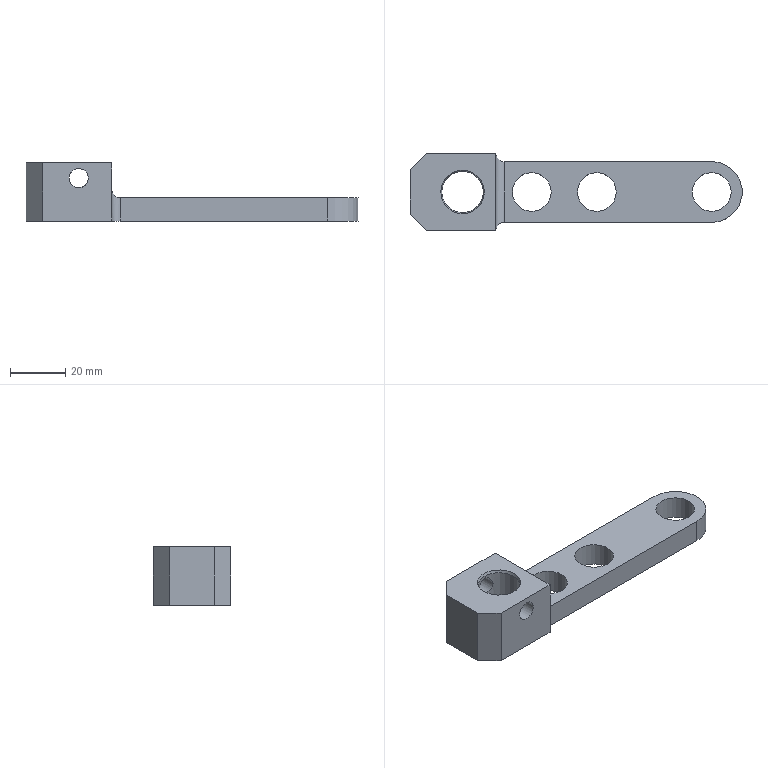NC program | NX | posted with a generic post | part box 120 x 28 x 21 mm
Lines 1 to 1650 of 1970, first 1501 of 1628 lines:
N10 G17 G21 G94 G90
(低壁铣光面 , TOOL : D50面刀)
N12 T01 M6
N14 G53
N16 G17 G0 G90 X87.971 Y-1.5 B0. C0. S3000 M3
N18 G43 Z20. H1
N20 Z3.
N22 G94 G1 Z0. F800.
N24 X84.969
N26 X-85.
N28 X-88.
N30 Z3.
N32 G0 Z20.
N34 M5
(动态粗 , TOOL : D10-30-D10-75-3T-粗)
N36 T02 M6
N38 G53
N40 G17 G0 G90 X73.022 Y0.609 B0. C0. S4500 M3
N42 G43 Z20. H2
N44 Z-20.5
N46 G94 G1 X72.997 Y0.614 Z-20.656 F2000.
N48 X72.973 Y0.619 Z-20.718
N50 X72.948 Y0.623 Z-20.763
N52 X72.924 Y0.628 Z-20.8
N54 X72.899 Y0.633 Z-20.831
N56 X72.875 Y0.637 Z-20.857
N58 X72.85 Y0.642 Z-20.88
N60 X72.826 Y0.647 Z-20.9
N62 X72.801 Y0.652 Z-20.918
N64 X72.776 Y0.656 Z-20.933
N66 X72.752 Y0.661 Z-20.947
N68 X72.727 Y0.666 Z-20.958
N70 X72.703 Y0.671 Z-20.968
N72 X72.678 Y0.675 Z-20.977
N74 X72.654 Y0.68 Z-20.984
N76 X72.629 Y0.685 Z-20.99
N78 X72.605 Y0.69 Z-20.994
N80 X72.58 Y0.694 Z-20.997
N82 X72.556 Y0.699 Z-20.999
N84 X72.531 Y0.704 Z-21.
N86 X71.2 Y0.961
N88 G3 X70. Y0.026 R1.01
N90 X69.81 Y-3.845 R27.515
N92 G1 X69.787 Y-13.98
N94 G2 X66.969 Y-18.352 R5.717
N96 X62.833 Y-19.626 R9.695
N98 X57.048 Y-19.797 R62.046
N100 G1 X53.763 Y-19.8
N102 X-63.71 Y-19.799
N104 G2 X-68.197 Y-17.198 R5.627
N106 X-69.611 Y-12.941 R9.369
N108 X-69.796 Y-7.546 R53.786
N110 G1 X-69.8 Y-3.631
N112 X-69.799 Y13.704
N114 G2 X-67.161 Y18.225 R5.629
N116 X-63.006 Y19.604 R9.352
N118 X-57.402 Y19.796 R53.99
N120 G1 X-53.502 Y19.8
N122 X63.711 Y19.799
N124 G2 X68.237 Y17.142 R5.634
N126 X69.62 Y12.869 R9.501
N128 X69.797 Y7.219 R58.798
N130 X69.761 Y0.495 R170.584
N132 G3 X69.601 Y-9.151 R167.76
N134 G2 X69.571 Y-12.9 R75.074
N136 X65.88 Y-18.221 R6.764
N138 X61.269 Y-19.44 R11.904
N140 X54.643 Y-19.598 R85.637
N142 G1 X51.838 Y-19.599
N144 X-62.334 Y-19.598
N146 G2 X-68.174 Y-15.959 R6.725
N148 X-69.423 Y-11.429 R11.621
N150 X-69.598 Y-4.774 R78.417
N152 G1 X-69.6 Y-1.804
N154 X-69.599 Y12.354
N156 G2 X-65.963 Y18.173 R6.722
N158 X-61.404 Y19.426 R11.654
N160 X-54.914 Y19.597 R77.61
N162 G1 X-51.944 Y19.599
N164 X62.354 Y19.598
N166 G2 X68.165 Y15.977 R6.718
N168 X69.418 Y11.484 R11.54
N170 X69.596 Y5.534 R68.242
N172 X69.453 Y-2.271 R158.679
N174 G3 X69.388 Y-11.581 R729.554
N176 G2 X65.029 Y-18.065 R7.462
N178 X60.202 Y-19.238 R13.485
N180 X52.706 Y-19.398 R103.38
N182 G1 X50.396 Y-19.399
N184 X-61.149 Y-19.398
N186 G2 X-68.097 Y-14.956 R7.496
N188 X-69.241 Y-10.152 R13.655
N190 X-69.397 Y-3.465 R93.67
N192 G1 X-69.4 Y-0.33
N194 G2 X-69.381 Y11.694 R885.31
N196 X-65.067 Y18.043 R7.455
N198 X-60.318 Y19.227 R13.283
N200 X-53.46 Y19.397 R88.823
N202 G1 X-50.55 Y19.399
N204 X61.155 Y19.398
N206 G2 X68.093 Y14.965 R7.492
N208 X69.24 Y10.175 R13.613
N210 X69.304 Y-0.538 R105.243
N212 G3 X69.183 Y-10.742 R552.283
N214 G2 X64.322 Y-17.885 R8.024
N216 X59.29 Y-19.037 R14.812
N218 X52.243 Y-19.197 R101.775
N220 G1 X49.108 Y-19.199
N222 X-28.994
N224 X-54.133 Y-19.2
N226 G2 X-60.954 Y-19.169 R221.811
N228 X-67.876 Y-14.335 R8.015
N230 X-69.032 Y-9.347 R14.712
N232 X-69.197 Y-2.196 R100.061
N234 G1 X-69.199 Y0.939
N236 G2 X-69.176 Y10.854 R546.259
N238 X-64.287 Y17.898 R8.025
N240 X-59.235 Y19.041 R14.939
N242 X-53.999 Y19.2 R95.861
N244 G1 X-27.434 Y19.199
N246 X59.971
N248 G2 X64.719 Y18.005 R8.632
N250 X68.318 Y13.208 R8.711
N252 X69.111 Y8.109 R19.175
N254 X69.063 Y-2.125 R148.538
N256 G1 X68.98 Y-9.982
N258 G2 X63.699 Y-17.695 R8.496
N260 X58.626 Y-18.825 R15.763
N262 X51.415 Y-18.996 R101.599
N264 G1 X48.61 Y-18.999
N266 X-27.504
N268 X-27.756 Y-19.033
N270 G3 X-28.471 Y-19.876 R1.001
N272 X-28.172 Y-20.72 Z-20.954 R1.046
N274 G1 X-27.475 Y-21.528 Z-20.9
N276 X-27.273 Y-21.759 F15000.
N278 X-27.083 Y-22.
N280 G2 X-27.834 Y-23.531 R1.008
N282 X-28.943 Y-22.898 R1.
N284 G1 X-29.388 Y-21.714
N286 X-29.623 Y-21.096 Z-20.933 F2000.
N288 X-29.848 Y-20.475 Z-20.966
N290 G2 X-29.818 Y-19.818 Z-21. R1.001
N292 X-28.994 Y-19.199 R1.001
N294 G1 X-27.938 Y-19.09
N296 G2 X-26.621 Y-18.919 R4.238
N298 X-21.798 Y-18.879 R444.97
N300 G1 X49.642 Y-18.878
N302 G3 X58.054 Y-18.732 R139.77
N304 X63.151 Y-17.71 R16.77
N306 X68.701 Y-10.494 R8.625
N308 X68.889 Y-6.106 R39.918
N310 G2 X69.06 Y3.055 R798.502
N312 G3 X68.819 Y10.051 R60.315
N314 X67.291 Y14.975 R12.294
N316 X61.091 Y18.896 R8.167
N318 X56.522 Y19.076 R39.1
N320 G1 X53.552 Y19.079
N322 X-27.799 Y19.08
N324 X-27.933 Y19.089
N326 G2 X-28.589 Y19.763 R1.001
N328 G1 X-29.11 Y21.687 Z-20.9
N330 X-29.229 Y22.113 F15000.
N332 X-29.331 Y22.544
N334 G2 X-27.933 Y23.573 R1.
N336 X-27.243 Y22.601 R1.031
N338 X-27.868 Y21.689 R1.001
N340 G1 X-28.045 Y21.618
N342 X-29.332 Y21.093 Z-20.97 F2000.
N344 G3 X-29.766 Y20.689 Z-21. R1.004
N346 X-28.999 Y19.2 R1.
N348 X-26.697 Y18.951 R76.002
N350 X-19.829 Y18.879 R185.542
N352 G1 X54.556 Y18.878
N354 G2 X60.088 Y18.752 R67.139
N356 X65.54 Y16.41 R8.839
N358 X68.273 Y11.314 R10.082
N360 X68.83 Y5.801 R27.486
N362 X68.728 Y-3.168 R222.735
N364 X68.582 Y-9.247 R118.626
N366 X66.842 Y-14.337 R9.723
N368 X61.648 Y-17.828 R9.71
N370 X56.18 Y-18.593 R22.544
N372 X46.656 Y-18.679 R288.01
N374 G1 X-21.741
N376 G3 X-26.918 Y-18.774 R68.031
N378 G1 X-27.744 Y-19.028
N380 G2 X-25.274 Y-18.606 R6.814
N382 X-19.998 Y-18.559 R311.969
N384 G1 X48.187 Y-18.558
N386 G3 X57.064 Y-18.414 R155.765
N388 X62.333 Y-17.402 R17.938
N390 X68.245 Y-10.195 R9.13
N392 X68.566 Y-5.756 R28.676
N394 X68.724 Y4.574 R587.278
N396 X68.293 Y10.43 R34.444
N398 X66.104 Y15.427 R10.805
N400 X60.517 Y18.472 R8.932
N402 X55.759 Y18.75 R31.579
N404 G1 X51.739 Y18.759
N406 X-20.312 Y18.76
N408 G2 X-26.885 Y18.863 R106.821
N410 X-27.938 Y19.09 R3.126
N412 G3 X-25.2 Y18.635 R8.455
N414 X-17.999 Y18.56 R207.111
N416 G1 X52.756 Y18.558
N418 G2 X58.888 Y18.422 R78.525
N420 X63.769 Y16.905 R10.593
N422 X67.642 Y11.613 R9.54
N424 X68.46 Y6.14 R21.211
N426 X68.42 Y-2.591 R148.221
N428 X68.213 Y-8.564 R82.081
N430 X66.489 Y-13.668 R10.653
N432 X61.086 Y-17.444 R9.954
N434 X55.625 Y-18.255 R22.265
N436 X45.337 Y-18.359 R265.527
N438 G1 X-19.941
N440 G3 X-25.829 Y-18.468 R82.64
N442 X-26.695 Y-18.639 R2.859
N444 X-27.133 Y-19.103 R1.007
N446 G1 X-27.464 Y-19.82
N448 X-28.299 Y-21.629 Z-20.9
N450 X-28.424 Y-21.903 F15000.
N452 X-28.558 Y-22.172
N454 G2 X-28.937 Y-22.522 R1.017
N456 G1 X-29.135 Y-22.627
N458 X-29.339 Y-22.722
N460 G2 X-30.664 Y-21.705 R1.
N462 X-30.147 Y-20.894 Z-20.95 R1.044 F2000.
N464 G1 X-29.327 Y-20.337 Z-21.
N466 X-27.216 Y-18.903
N468 G2 X-26.361 Y-18.515 R5.645
N470 X-23.232 Y-18.264 R16.51
N472 G1 X-17.569 Y-18.238
N474 X47.341
N476 G3 X56.234 Y-18.089 R155.919
N478 X61.609 Y-17.076 R18.781
N480 X67.831 Y-9.742 R9.577
N482 X68.253 Y-4.862 R27.855
N484 X68.363 Y5.186 R245.433
N486 X67.704 Y10.775 R24.736
N488 X64.472 Y16.067 R9.964
N490 X59.33 Y18.176 R10.222
N492 X53.956 Y18.433 R41.143
N494 G1 X50.101 Y18.439
N496 X-18.661 Y18.44
N498 G2 X-25.746 Y18.566 R107.934
N500 X-26.846 Y18.732 R5.693
N502 X-26.119 Y20.595 R1.
N504 G1 X-24.223 Y19.982 Z-20.9
N506 G3 X-23.676 Y21.903 R1. F15000.
N508 G1 X-23.959 Y22.001
N510 X-24.246 Y22.089
N512 G3 X-24.89 Y22.003 R1.007
N514 G1 X-26.413 Y21.241
N516 X-27.494 Y20.694 Z-20.961 F2000.
N518 G3 X-27.953 Y20.088 Z-21. R1.
N520 X-27.289 Y18.884 R1.
N522 X-26.175 Y18.532 R9.502
N524 X-22.01 Y18.263 R27.335
N526 G1 X-16.543 Y18.24
N528 X51.156 Y18.238
N530 G2 X57.798 Y18.102 R92.333
N532 X62.729 Y16.769 R12.135
N534 X67.208 Y11.202 R9.727
N536 X68.108 Y5.727 R20.279
N538 X68.093 Y-2.926 R135.301
N540 X67.796 Y-8.404 R47.795
N542 X65.497 Y-13.896 R10.604
N544 X60.044 Y-17.214 R10.683
N546 X54.449 Y-17.948 R25.14
N548 X43.32 Y-18.038 R341.418
N550 G1 X-18.995 Y-18.039
N552 G3 X-25.041 Y-18.169 R79.601
N554 X-26.295 Y-18.413 R4.296
N556 G1 X-26.673 Y-18.626
N558 G2 X-25.002 Y-18.098 R3.475
N560 X-19.801 Y-17.923 R51.666
N562 G1 X-16.758 Y-17.919
N564 X48.502 Y-17.914
N566 G3 X56.282 Y-17.7 R97.674
N568 X61.705 Y-16.432 R16.824
N570 X67.419 Y-9.347 R9.918
N572 X67.934 Y-4.281 R26.306
N574 X67.994 Y5.332 R152.676
N576 X67.115 Y10.916 R20.724
N578 X62.077 Y16.819 R9.708
N580 X57.141 Y17.988 R13.737
N582 X50.799 Y18.118 R96.817
N584 G1 X48.549 Y18.119
N586 X-17.267 Y18.12
N588 G2 X-24.696 Y18.255 R115.566
N590 X-26.617 Y18.594 R6.877
N592 X-26.061 Y20.468 R1.
N594 G1 X-25.807 Y20.418 Z-20.987
N596 X-25.559 Y20.341 Z-20.974
N598 X-24.148 Y19.917 Z-20.9
N600 G3 X-23.446 Y21.765 R1. F15000.
N602 G1 X-23.821 Y21.966
N604 G3 X-24.736 Y21.874 R1.001
N606 G1 X-25.946 Y21.083
N608 X-26.978 Y20.403 Z-20.962 F2000.
N610 G3 X-27.362 Y19.773 Z-21. R1.001
N612 X-26.868 Y18.737 R1.
N614 X-24.978 Y18.16 R4.359
N616 X-19.468 Y17.93 R49.854
N618 G1 X-14.398 Y17.92
N620 X49.801 Y17.918
N622 G2 X56.833 Y17.782 R103.44
N624 X61.856 Y16.54 R13.461
N626 X66.82 Y10.686 R9.999
N628 X67.766 Y5.099 R20.278
N630 X67.598 Y-6.505 R119.238
N632 X66.285 Y-11.588 R13.689
N634 X60.445 Y-16.551 R10.225
N636 X54.763 Y-17.569 R20.721
N638 X46.276 Y-17.717 R157.879
N640 G1 X40.276 Y-17.718
N642 X-17.645 Y-17.72
N644 G3 X-24.193 Y-17.851 R92.996
N646 X-25.871 Y-18.165 R5.563
N648 G1 X-25.948 Y-18.211
N650 G3 X-26.363 Y-18.935 R1.002
N652 G1 X-26.395 Y-19.282
N654 X-26.573 Y-21.267 Z-20.9
N656 X-26.6 Y-21.586 F15000.
N658 X-26.64 Y-21.903
N660 G2 X-27.109 Y-22.542 R1.003
N662 G1 X-27.327 Y-22.67
N664 X-27.551 Y-22.788
N666 G2 X-28.909 Y-21.699 R1.
N668 X-28.628 Y-21.145 Z-20.932 R1.093 F2000.
N670 G1 X-27.758 Y-20.097 Z-21.
N672 X-26.533 Y-18.622
N674 G2 X-24.925 Y-17.885 R3.03
N676 X-20.772 Y-17.619 R27.047
N678 G1 X-14.898 Y-17.599
N680 X48.316 Y-17.592
N682 G3 X55.959 Y-17.336 R84.299
N684 X61.523 Y-15.895 R16.268
N686 X67.034 Y-8.88 R10.257
N688 X67.616 Y-3.657 R25.896
N690 X67.614 Y5.4 R105.018
N692 X66.509 Y11. R18.349
N694 X59.147 Y17.252 R10.06
N696 X53.917 Y17.767 R25.601
N698 G1 X47.032 Y17.799
N700 X-15.347 Y17.8
N702 G2 X-23.569 Y17.925 R151.062
N704 X-26.183 Y18.352 R9.887
N706 G1 X-26.537 Y18.55
N708 G3 X-24.43 Y17.875 R4.866
N710 X-18.668 Y17.613 R48.879
N712 G1 X-12.509 Y17.6
N714 X48.506 Y17.598
N716 G2 X55.958 Y17.46 R114.528
N718 X61.128 Y16.25 R14.546
N720 X66.431 Y10.206 R10.268
N722 X67.426 Y4.446 R20.398
N724 X67.252 Y-6.017 R89.365
N726 X65.784 Y-11.302 R13.855
N728 X59.797 Y-16.232 R10.572
N730 X54.097 Y-17.241 R21.36
N732 X44.29 Y-17.398 R178.207
N734 G1 X-14.888 Y-17.399
N736 G3 X-23.092 Y-17.511 R153.117
N738 X-25.629 Y-17.97 R8.308
N740 G1 X-25.807 Y-18.081
N742 G3 X-26.168 Y-18.71 R1.004
N744 G1 X-26.256 Y-19.291
N746 X-26.553 Y-21.262 Z-20.9
N748 X-26.601 Y-21.604 F15000.
N750 X-26.666 Y-21.944
N752 G2 X-26.967 Y-22.412 R1.012
N754 G1 X-27.272 Y-22.662
N756 G2 X-28.8 Y-21.693 R1.
N758 X-28.498 Y-21.088 Z-20.934 R1.079 F2000.
N760 G1 X-27.638 Y-20.107 Z-21.
N762 X-26.083 Y-18.333
N764 G2 X-24.823 Y-17.676 R2.213
N766 X-20.857 Y-17.318 R20.383
N768 X-13.773 Y-17.279 R605.408
N770 G1 X48.179 Y-17.269
N772 G3 X55.52 Y-16.983 R76.095
N774 X61.194 Y-15.435 R16.184
N776 X66.65 Y-8.448 R10.56
N778 X67.292 Y-3.157 R25.169
N780 X67.229 Y5.358 R77.908
N782 X65.894 Y11.039 R16.909
N784 X58.747 Y16.853 R10.338
N786 X53.54 Y17.433 R24.327
N788 X45.59 Y17.479 R578.396
N790 G1 X-13.997 Y17.48
N792 G2 X-22.765 Y17.611 R163.509
N794 X-25.754 Y18.101 R11.318
N796 G1 X-25.913 Y18.185
N798 G2 X-25.717 Y19.95 R1.
N800 X-24.995 Y19.953 Z-20.963 R1.067
N802 G1 X-23.786 Y19.614 Z-20.9
N804 X-23.398 Y19.517 F15000.
N806 G3 X-22.743 Y21.355 R1.
N808 X-23.199 Y21.594 R1.725
N810 X-24.029 Y21.458 R1.002
N812 G1 X-25.185 Y20.675
N814 X-26.227 Y19.964 Z-20.963 F2000.
N816 G3 X-26.598 Y19.354 Z-21. R1.001
N818 X-26.106 Y18.306 R1.
N820 X-24.385 Y17.663 R3.881
N822 X-19.329 Y17.313 R33.113
N824 G1 X-10.979 Y17.28
N826 X45.556 Y17.279
N828 G2 X54.545 Y17.177 R201.846
N830 X59.793 Y16.22 R17.499
N832 X66.064 Y9.686 R10.519
N834 X67.08 Y3.93 R20.473
N836 X66.892 Y-5.675 R68.153
N838 X65.227 Y-11.132 R13.735
N840 X59.111 Y-15.933 R10.932
N842 X53.302 Y-16.923 R22.463
N844 X44.634 Y-17.078 R162.319
N846 G1 X34.314 Y-17.079
N848 X-15.32 Y-17.08
N850 G3 X-22.776 Y-17.224 R110.442
N852 X-25.372 Y-17.743 R8.359
N854 X-25.809 Y-18.081 R3.883
N856 G2 X-24.393 Y-17.384 R2.634
N858 X-20.164 Y-17.001 R22.157
N860 X-12.813 Y-16.959 R609.767
N862 G1 X48.06 Y-16.945
N864 G3 X55.278 Y-16.608 R67.044
N866 X61.026 Y-14.895 R15.745
N868 X66.294 Y-7.941 R10.861
N870 X66.979 Y-2.294 R25.868
N872 X66.809 Y5.543 R57.325
N874 X65.159 Y11.258 R15.389
N876 X58.279 Y16.477 R10.619
N878 X52.822 Y17.108 R24.692
N880 X43.603 Y17.159 R528.663
N882 G1 X-12.887 Y17.16
N884 G2 X-21.915 Y17.29 R179.27
N886 X-25.232 Y17.8 R13.491
N888 X-25.795 Y18.07 R2.99
N890 X-24.622 Y19.686 R1.
N892 G1 X-23.875 Y19.207
N894 X-23.46 Y18.94 Z-20.975
N896 X-23.04 Y18.679 Z-20.95
N898 G3 X-22.079 Y18.686 Z-20.9 R0.999
N900 X-21.911 Y20.312 R1. F15000.
N902 X-22.3 Y20.597 R1.541
N904 X-22.995 Y20.651 R1.005
N906 G1 X-24.455 Y20.232
N908 X-25.628 Y19.89 Z-20.961 F2000.
N910 G3 X-26.186 Y19.388 Z-21. R1.
N912 X-25.946 Y18.201 R1.
N914 X-24.446 Y17.488 R3.067
N916 X-20.211 Y17.037 R22.141
N918 X-9.914 Y16.96 R387.709
N920 G1 X46.172 Y16.958
N922 G2 X54.359 Y16.818 R136.018
N924 X59.733 Y15.673 R16.532
N926 X65.722 Y9.123 R10.793
N928 X66.742 Y3.26 R20.935
N930 X66.518 Y-5.427 R53.423
N932 X64.595 Y-11.081 R13.466
N934 X58.469 Y-15.626 R11.289
N936 X52.595 Y-16.601 R23.412
N938 X43.777 Y-16.758 R164.422
N940 G1 X-12.803 Y-16.759
N942 G3 X-21.679 Y-16.876 R177.288
N944 X-24.851 Y-17.395 R11.802
N946 X-25.543 Y-17.848 R1.747
N948 G2 X-24.129 Y-17.127 R2.71
N950 X-19.965 Y-16.697 R20.667
N952 X-11.838 Y-16.639 R422.525
N954 G1 X46.742
N956 G3 X54.207 Y-16.333 R84.296
N958 X60.026 Y-14.804 R17.306
N960 X65.952 Y-7.404 R11.133
N962 X66.648 Y-1.728 R25.667
N964 X66.363 Y5.757 R44.317
N966 X64.312 Y11.567 R14.192
N968 X57.609 Y16.162 R10.975
N970 X52.165 Y16.782 R25.717
N972 X42.805 Y16.839 R470.105
N974 G1 X-11.747 Y16.841
N976 G2 X-21.202 Y16.973 R191.97
N978 X-24.871 Y17.536 R14.736
N980 X-25.752 Y18.031 R2.137
N982 G3 X-24.143 Y17.229 R3.322
N984 X-19.703 Y16.728 R22.056
N986 X-8.414 Y16.639 R383.664
N988 G1 X45.041 Y16.638
N990 G2 X53.619 Y16.496 R146.744
N992 X59.049 Y15.39 R17.493
N994 X65.367 Y8.614 R11.026
N996 X66.402 Y2.631 R21.243
N998 X66.121 Y-5.302 R42.372
N1000 X63.893 Y-11.108 R13.11
N1002 X57.804 Y-15.33 R11.675
N1004 X51.91 Y-16.28 R24.466
N1006 X42.715 Y-16.434 R173.357
N1008 G1 X34.315 Y-16.439
N1010 X-13.505 Y-16.44
N1012 G3 X-21.411 Y-16.583 R131.271
N1014 X-24.58 Y-17.143 R11.604
N1016 X-25.125 Y-17.464 R1.638
N1018 X-25.382 Y-17.965 R1.012
N1020 G1 X-25.601 Y-19.109
N1022 X-25.975 Y-21.067 Z-20.9
N1024 G2 X-26.112 Y-21.558 R1.669 F15000.
N1026 X-26.649 Y-22.101 R1.571
N1028 X-28.038 Y-21.622 R1.
N1030 X-27.81 Y-20.488 Z-20.962 R1.027 F2000.
N1032 G1 X-27.307 Y-19.916 Z-21.
N1034 X-25.341 Y-17.682
N1036 G2 X-23.984 Y-16.897 R2.438
N1038 X-20.068 Y-16.407 R17.812
N1040 X-10.818 Y-16.32 R274.581
N1042 G1 X46.742 Y-16.319
N1044 G3 X53.988 Y-15.963 R74.94
N1046 X59.897 Y-14.271 R16.816
N1048 X65.577 Y-7.01 R11.345
N1050 X66.313 Y-1.009 R25.21
N1052 X65.881 Y6.03 R34.936
N1054 X63.34 Y11.935 R13.242
N1056 X56.899 Y15.86 R11.405
N1058 X51.242 Y16.466 R27.839
N1060 X42.292 Y16.519 R540.119
N1062 G1 X-10.532 Y16.52
N1064 G2 X-20.439 Y16.651 R213.822
N1066 X-24.428 Y17.235 R16.71
N1068 X-25.494 Y17.805 R2.496
N1070 G3 X-23.822 Y16.96 R3.521
N1072 X-19.269 Y16.419 R22.139
N1074 X-7.229 Y16.319 R372.609
N1076 G1 X44.236 Y16.318
N1078 G2 X52.919 Y16.174 R151.221
N1080 X58.458 Y15.074 R18.275
N1082 X65.015 Y8.112 R11.244
N1084 X66.061 Y1.922 R21.583
N1086 X65.675 Y-5.403 R33.609
N1088 X62.828 Y-11.534 R12.511
N1090 X56.756 Y-15.15 R12.376
N1092 X51.794 Y-15.928 R25.856
N1094 G1 X50.962 Y-16.081
N1096 X49. Y-16.2
N1098 X-19.363 Y-16.205
N1100 G3 X-23.735 Y-16.692 R19.421
N1102 X-25.003 Y-17.297 R2.826
N1104 G1 X-25.033 Y-17.331
N1106 G3 X-25.027 Y-18.71 R1.1
N1108 X-23.923 Y-19.093 Z-20.938 R1.133
N1110 G1 X-23.168 Y-18.985 Z-20.9
N1112 X-21.127 Y-18.693 F15000.
N1114 X-19.154 Y-18.411 Z-21. F2000.
N1116 G3 X-18.441 Y-18.132 R1.236
N1118 X-19.16 Y-16.2 R1.1
N1120 X-22.332 Y-16.282 R26.908
N1122 X-24.69 Y-16.972 R6.037
N1124 X-25.184 Y-17.531 R2.235
N1126 G2 X-23.819 Y-16.538 R2.223
N1128 X-21.241 Y-16.2 R6.76
N1130 G3 X-23.175 Y-16.272 R11.071
N1132 X-24.707 Y-16.911 R3.159
N1134 G1 X-24.912 Y-17.169
N1136 G2 X-23.741 Y-16.367 R2.002
N1138 X-22.533 Y-16.2 R2.885
N1140 G3 X-24.449 Y-16.624 R3.185
N1142 X-24.75 Y-16.955 R3.169
N1144 G2 X-23.141 Y-16.2 R1.8
N1146 G3 X-24.477 Y-16.604 R1.722
N1148 G1 X-24.63 Y-16.796
N1150 G2 X-23.499 Y-16.2 R1.306
N1152 G3 X-24.47 Y-16.596 R1.148
N1154 X-24.66 Y-17.577 R1.001
N1156 G1 X-24.566 Y-17.848
N1158 X-23.917 Y-19.732 Z-20.9
N1160 G2 X-24.205 Y-20.928 R1.026 F15000.
N1162 G1 X-24.333 Y-21.012
N1164 X-24.47 Y-21.08
N1166 X-25.239 Y-21.379
N1168 X-26.013 Y-21.667
N1170 G2 X-28.019 Y-22.073 R8.521
N1172 X-32.369 Y-22.278 R53.35
N1174 G1 X-50.83 Y-22.371
N1176 G2 X-51.654 Y-21.944 R1.001
N1178 G1 X-51.823 Y-21.703
N1180 X-52.966 Y-20.07 Z-21. F2000.
N1182 X-53.161 Y-19.785
N1184 X-53.37 Y-19.51
N1186 G3 X-54.001 Y-19.2 R1.005
N1188 X-58.986 Y-19.004 R43.03
N1190 G2 X-63.131 Y-18.321 R10.577
N1192 X-67.849 Y-13.321 R8.685
N1194 X-68.863 Y-8.114 R17.25
N1196 X-68.998 Y-0.271 R139.467
N1198 X-68.977 Y9.984 R692.379
N1200 X-63.716 Y17.685 R8.49
N1202 X-58.496 Y18.834 R15.908
N1204 G1 X-55.41 Y18.983
N1206 X-55.013 Y19.1
N1208 X-54.087 Y19.191
N1210 G3 X-55.527 Y18.955 R5.334
N1212 G2 X-59.179 Y18.636 R235.177
N1214 G3 X-64.174 Y17.231 R13.721
N1216 X-68.7 Y10.484 R8.58
N1218 X-68.875 Y6.08 R38.287
N1220 X-68.801 Y-6.789 R425.011
N1222 X-68.086 Y-12.052 R22.091
N1224 X-64.729 Y-17.091 R9.307
N1226 X-59.826 Y-18.774 R9.44
N1228 X-55.505 Y-18.965 R256.415
N1230 G1 X-55.387 Y-18.987
N1232 G2 X-55.965 Y-20.901 R-1.
N1234 G1 X-56.559 Y-20.707
N1236 X-58.02 Y-20.234 Z-20.923
N1238 G3 X-58.472 Y-20.222 Z-20.9 R1.015
N1240 X-58.558 Y-22.158 R1. F15000.
N1242 G1 X-58.301 Y-22.237
N1244 X-58.041 Y-22.303
N1246 G3 X-57.46 Y-22.213 R1.01
N1248 G1 X-55.899 Y-21.455
N1250 X-54.809 Y-20.921 Z-20.961 F2000.
N1252 G3 X-54.343 Y-20.323 Z-21. R1.
N1254 X-55.016 Y-19.1 R1.
N1256 X-57.274 Y-18.738 R8.023
N1258 G2 X-61.101 Y-18.309 R22.726
N1260 X-67.433 Y-12.77 R8.957
N1262 X-68.522 Y-7.443 R17.326
N1264 X-68.678 Y0.609 R129.207
N1266 X-68.614 Y8.693 R209.886
N1268 X-67.456 Y13.357 R10.795
N1270 X-62.238 Y17.635 R9.26
N1272 X-57.716 Y18.525 R19.082
N1274 G3 X-56.151 Y18.726 R9.529
N1276 G1 X-56.123 Y18.737
N1278 G3 X-55.528 Y19.503 R1.001
N1280 G1 X-55.52 Y19.731 Z-20.989
N1282 X-55.544 Y19.957 Z-20.977
N1284 X-55.712 Y21.485 Z-20.9
N1286 X-55.803 Y22.305 F15000.
N1288 G3 X-57.283 Y23.069 R1.
N1290 G1 X-57.535 Y22.931
N1292 X-57.778 Y22.78
N1294 G3 X-57.21 Y20.991 R1.
N1296 G1 X-56.4 Y20.965 Z-20.941 F2000.
N1298 X-55.591 Y20.928 Z-20.981
N1300 X-55.409 Y20.892 Z-20.991
N1302 X-55.237 Y20.824 Z-21.
N1304 G2 X-55.41 Y18.98 R1.
N1306 G3 X-56.35 Y18.657 R12.614
N1308 G2 X-59.522 Y18.161 R92.78
N1310 G3 X-64.542 Y16.233 R12.254
N1312 X-68.242 Y10.181 R9.117
N1314 X-68.548 Y5.532 R28.745
N1316 X-68.459 Y-6.272 R286.401
N1318 X-67.63 Y-11.683 R21.029
N1320 X-63.577 Y-17.022 R9.399
N1322 X-59.013 Y-18.44 R11.2
N1324 G2 X-56.097 Y-18.763 R46.889
N1326 G1 X-56.04 Y-18.782
N1328 G2 X-56.736 Y-20.656 R1.
N1330 G1 X-56.827 Y-20.626
N1332 X-58.662 Y-20.033 Z-20.903
N1334 X-58.724 Y-20.017 Z-20.9
N1336 G3 X-59.211 Y-21.953 R1. F15000.
N1338 G1 X-58.871 Y-22.063
N1340 X-58.527 Y-22.157
N1342 G3 X-57.935 Y-22.067 R1.009
N1344 G1 X-56.384 Y-21.309
N1346 X-55.294 Y-20.771 Z-20.961 F2000.
N1348 G3 X-54.83 Y-20.173 Z-21. R1.
N1350 X-55.504 Y-18.951 R1.
N1352 X-57.726 Y-18.422 R9.962
N1354 G2 X-61.65 Y-17.562 R17.287
N1356 X-67.206 Y-11.788 R9.509
N1358 X-68.216 Y-6.334 R19.143
N1360 X-68.357 Y2.514 R159.442
N1362 X-68.205 Y8.554 R68.921
N1364 X-66.463 Y13.699 R10.598
N1366 X-61.27 Y17.395 R9.966
N1368 X-57.268 Y18.286 R30.445
N1370 G3 X-56.088 Y18.751 R3.143
N1372 G2 X-57.982 Y18.068 R5.211
N1374 G3 X-62.167 Y16.863 R20.487
N1376 X-67.833 Y9.696 R9.585
N1378 X-68.223 Y4.648 R27.749
N1380 X-68.11 Y-5.91 R192.596
N1382 X-67.156 Y-11.39 R19.901
N1384 X-60.101 Y-17.809 R9.725
N1386 X-56.782 Y-18.476 R101.747
N1388 G2 X-56.022 Y-18.787 R2.413
N1390 G3 X-57.912 Y-18.114 R5.908
N1392 G2 X-61.855 Y-16.869 R17.322
N1394 X-66.968 Y-10.855 R10.111
N1396 X-67.907 Y-5.295 R21.039
N1398 X-67.937 Y6.851 R147.556
N1400 X-66.834 Y11.785 R13.665
N1402 X-61.422 Y16.786 R9.919
N1404 X-57.765 Y17.907 R31.027
N1406 G3 X-57.056 Y18.187 R2.653
N1408 X-56.667 Y18.871 R1.003
N1410 G1 X-56.618 Y19.302
N1412 X-56.394 Y21.282 Z-20.9
N1414 X-56.36 Y21.613 F15000.
N1416 X-56.309 Y21.941
N1418 G2 X-55.896 Y22.518 R1.005
N1420 G1 X-55.655 Y22.681
N1422 X-55.407 Y22.831
N1424 G2 X-54.007 Y21.702 R1.
N1426 X-54.276 Y21.211 Z-20.928 R1.105 F2000.
N1428 G1 X-55.19 Y20.116 Z-21.
N1430 X-56.4 Y18.667
N1432 G2 X-56.888 Y18.324 R1.768
N1434 X-58.058 Y17.755 R2.854
N1436 G3 X-61.76 Y16.452 R27.065
N1438 X-67.457 Y9.12 R10.074
N1440 X-67.896 Y3.912 R27.606
N1442 X-67.751 Y-5.655 R134.782
N1444 X-66.651 Y-11.196 R18.798
N1446 X-60.096 Y-17.349 R10.255
N1448 G1 X-57.04 Y-18.245
N1450 X-56.906 Y-18.312
N1452 G2 X-58.044 Y-19.956 R1.
N1454 G1 X-58.454 Y-19.689
N1456 X-59.831 Y-18.801 Z-20.918
N1458 X-59.992 Y-18.729 Z-20.909
N1460 X-60.164 Y-18.685 Z-20.9
N1462 G3 X-60.789 Y-20.554 R1. F15000.
N1464 G1 X-60.515 Y-20.704
N1466 X-60.235 Y-20.844
N1468 G3 X-59.718 Y-20.896 R1.016
N1470 G1 X-57.945 Y-20.606
N1472 X-56.716 Y-20.4 Z-20.963 F2000.
N1474 G3 X-56.115 Y-19.988 Z-21. R1.001
N1476 X-56.471 Y-18.547 R1.
N1478 X-58.509 Y-17.664 R8.389
N1480 G2 X-62.623 Y-15.773 R14.92
N1482 X-66.763 Y-9.824 R10.905
N1484 X-67.604 Y-4.14 R23.824
N1486 X-67.592 Y6.236 R111.857
N1488 X-66.41 Y11.321 R14.191
N1490 X-61.132 Y16.364 R10.43
N1492 X-57.916 Y17.609 R65.295
N1494 G3 X-57.055 Y18.187 R2.806
N1496 G2 X-58.756 Y17.204 R4.711
N1498 G3 X-62.554 Y15.384 R19.837
N1500 X-67.087 Y8.587 R10.553
N1502 X-67.569 Y3.157 R27.796
N1504 X-67.361 Y-5.717 R92.895
N1506 X-66.016 Y-11.306 R17.171
N1508 X-60.124 Y-16.888 R10.889
N1510 G2 X-57.404 Y-17.963 R155.347
N1512 G1 X-57.16 Y-18.101
N1514 G2 X-58.323 Y-19.726 R1.
N1516 G1 X-58.556 Y-19.576
N1518 X-59.93 Y-18.695 Z-20.918
N1520 X-60.095 Y-18.623 Z-20.909
N1522 X-60.269 Y-18.58 Z-20.9
N1524 G3 X-61.043 Y-20.343 R1. F15000.
N1526 G1 X-60.663 Y-20.643
N1528 G3 X-59.882 Y-20.758 R1.003
N1530 G1 X-58.369 Y-20.355
N1532 X-57.2 Y-20.039 Z-20.961 F2000.
N1534 G3 X-56.628 Y-19.538 Z-21. R1.
N1536 X-56.89 Y-18.323 R1.
N1538 X-58.471 Y-17.391 R5.245
N1540 G2 X-62.211 Y-15.411 R18.55
N1542 X-66.263 Y-9.763 R11.085
N1544 X-67.256 Y-3.879 R22.483
N1546 X-67.235 Y5.82 R83.379
N1548 X-65.893 Y11.093 R14.214
N1550 X-60.999 Y15.901 R11.072
N1552 G1 X-58.112 Y17.293
N1554 G3 X-57.526 Y17.801 R8.276
N1556 G2 X-58.268 Y17.174 R6.421
N1558 X-60.976 Y15.751 R206.249
N1560 G3 X-66.788 Y7.767 R11.275
N1562 X-67.245 Y2.019 R30.981
N1564 X-66.941 Y-5.906 R65.052
N1566 X-65.239 Y-11.656 R15.824
N1568 X-60.152 Y-16.432 R11.753
N1570 G2 X-57.668 Y-17.684 R45.819
N1572 G1 X-57.239 Y-18.036
N1574 G3 X-59.11 Y-16.781 R8.466
N1576 G2 X-63.102 Y-13.954 R15.951
N1578 X-66.327 Y-7.803 R12.761
N1580 X-67. Y-1.58 R31.758
N1582 X-67.025 Y5.489 R244.453
N1584 X-66.028 Y9.475 R23.543
N1586 X-61.058 Y15.345 R11.657
N1588 G3 X-58.516 Y16.842 R110.848
N1590 G1 X-57.941 Y17.413
N1592 G2 X-59.625 Y16.08 R6.271
N1594 G3 X-63.257 Y13.403 R17.944
N1596 X-66.435 Y7.519 R12.36
N1598 X-66.899 Y3.265 R17.058
N1600 G1 X-66.915 Y-5.65
N1602 G2 X-67.036 Y-6.128 R1.021
N1604 X-67.406 Y-6.532 Z-20.972 R1.437
N1606 G1 X-68.496 Y-7.474 Z-20.9
N1608 X-68.674 Y-7.627 F15000.
N1610 X-68.844 Y-7.789
N1612 G3 X-68.876 Y-9.048 R1.
N1614 G1 X-61.489 Y-18.671
N1616 G3 X-60.826 Y-19.053 R1.003
N1618 G1 X-59.683 Y-19.203
N1620 X-58.466 Y-19.358 Z-20.962 F2000.
N1622 G3 X-57.757 Y-19.124 Z-21. R1.001
N1624 X-57.699 Y-17.655 R1.
N1626 X-59.209 Y-16.557 R7.656
N1628 G2 X-62.989 Y-13.623 R16.857
N1630 X-66.151 Y-7.277 R13.515
N1632 X-66.695 Y-1.614 R26.282
N1634 G1 X-66.697 Y5.5
N1636 G2 X-65.154 Y10.221 R19.001
N1638 X-60.867 Y14.964 R13.038
N1640 G1 X-59.314 Y16.04
N1642 X-58.515 Y16.839
N1644 G2 X-60.798 Y14.873 R13.776
N1646 G3 X-65.144 Y9.799 R13.668
N1648 X-66.554 Y3.713 R13.749
N1650 X-66.587 Y-5.652 R573.286
N1652 G2 X-66.708 Y-6.13 R1.021
N1654 G1 X-66.876 Y-6.364 Z-20.986
N1656 X-67.062 Y-6.583 Z-20.971
N1658 X-67.97 Y-7.671 Z-20.9
N1660 X-68.673 Y-8.511 F15000.
N1662 G3 X-68.829 Y-9.536 R1.001
N1664 G1 X-68.294 Y-10.833
N1666 X-67.744 Y-12.123
N1668 G3 X-65.438 Y-15.413 R11.565
N1670 G1 X-62.189 Y-18.657
N1672 G3 X-61.569 Y-18.945 R1.006
N1674 G1 X-59.784 Y-19.101
N1676 X-58.58 Y-19.201 Z-20.961 F2000.
N1678 G3 X-57.869 Y-18.921 Z-21. R1.
N1680 X-57.858 Y-17.496 R1.
N1682 X-59.766 Y-16.002 R11.769
N1684 G2 X-63.988 Y-11.808 R14.734
N1686 X-66.319 Y-3.797 R15.884
N1688 X-66.369 Y5.491 R238.42
N1690 X-64.9 Y9.672 R21.164
N1692 G1 X-64.803 Y9.991
N1694 G2 X-63.162 Y12.348 R8.913
N1696 X-60.805 Y14.549 R21.443
N1698 G1 X-59.373 Y15.981
N1700 X-63.676 Y11.677
N1702 X-64.323 Y10.89
N1704 X-63.676 Y11.677
N1706 X-61.389 Y13.965
N1708 X-63.676 Y11.677
N1710 G3 X-64.803 Y9.991 R6.056
N1712 G1 X-65.809 Y6.96
N1714 G3 X-66.243 Y2.884 R16.852
N1716 G1 X-66.26 Y-5.641
N1718 G2 X-66.423 Y-6.188 R1.011
N1720 G1 X-67.05 Y-6.962 Z-20.95
N1722 X-67.689 Y-7.727 Z-20.9
N1724 X-68.343 Y-8.516 F15000.
N1726 G3 X-68.502 Y-9.524 R1.001
N1728 G1 X-68.179 Y-10.334
N1730 X-67.847 Y-11.139
N1732 G3 X-66.892 Y-12.877 R12.294
N1734 G1 X-65.763 Y-14.57
N1736 G3 X-63.769 Y-17.006 R21.746
N1738 G1 X-62.465 Y-18.381
N1740 G3 X-61.82 Y-18.69 R1.005
N1742 G1 X-60.053 Y-18.833
N1744 X-58.85 Y-18.925 Z-20.961 F2000.
N1746 G3 X-58.14 Y-18.641 Z-21. R1.
N1748 X-58.134 Y-17.22 R1.
N1750 X-60.233 Y-15.431 R18.443
N1752 G2 X-63.819 Y-11.504 R15.243
N1754 G1 X-64.324 Y-10.888
N1756 G2 X-65.236 Y-8.672 R7.808
N1758 X-66.023 Y-3.183 R18.928
N1760 X-66.042 Y5.491 R513.99
N1762 X-65.176 Y8.265 R41.822
N1764 X-64.943 Y9.533 R4.161
N1766 G3 X-65.177 Y8.236 R4.184
N1768 X-65.683 Y6.113 R70.955
N1770 X-65.927 Y1.97 R26.888
N1772 G1 X-65.933 Y-5.64
N1774 G2 X-66.189 Y-6.308 R1.005
N1776 G1 X-66.674 Y-6.744 Z-20.967
N1778 X-67.169 Y-7.169 Z-20.935
N1780 X-67.689 Y-7.62 Z-20.9
N1782 X-68.342 Y-8.191 F15000.
N1784 X-69.004 Y-8.751
N1786 X-69.202 Y-8.869
N1788 X-69.383 Y-9.01
N1790 G3 X-68.863 Y-10.696 R1.
N1792 G1 X-67.07 Y-11.044
N1794 X-65.881 Y-11.269 Z-20.961 F2000.
N1796 G3 X-65.146 Y-11.067 Z-21. R1.
N1798 X-64.805 Y-9.989 R1.
N1800 G2 X-65.327 Y-7.739 R12.108
N1802 X-65.713 Y-2.932 R26.339
N1804 X-65.716 Y5.488 R632.755
N1806 G3 X-65.203 Y7.429 R119.032
N1808 G1 X-65.176 Y8.24
N1810 G2 X-65.231 Y7.154 R34.006
N1812 G3 X-65.597 Y2.858 R21.064
N1814 G1 X-65.609 Y-5.652
N1816 G2 X-65.811 Y-6.255 R1.008
N1818 G1 X-66.434 Y-7.078
N1820 X-67.635 Y-8.668 Z-20.9
N1822 X-68.131 Y-9.323 F15000.
N1824 G2 X-69.492 Y-7.894 R-1.
N1826 X-68.056 Y-8.095 R1.011
N1828 G1 X-67.652 Y-8.658
N1830 X-66.862 Y-9.749 Z-20.968 F2000.
N1832 G3 X-66.324 Y-10.085 Z-21. R1.002
N1834 X-65.1 Y-9.013 R1.
N1836 G2 X-65.403 Y-2.402 R55.046
N1838 G1 X-65.396 Y5.087
N1840 G3 X-65.2 Y7.428 R8.206
N1842 G2 X-65.274 Y3.947 R107.738
N1844 G1 X-65.284 Y-5.703
N1846 G2 X-65.2 Y-7.999 R14.139
N1848 G1 Y6.179
N1850 Y-7.999
N1852 G3 X-64.805 Y-9.989 R6.056
N1854 X-63.677 Y-11.676 R6.072
N1856 X-59.545 Y-15.809 R23.851
N1858 G1 X-58.537 Y-16.817
N1860 X-63.677 Y-11.676
N1862 G3 X-64.422 Y-11.384 R1.003
N1864 G1 X-64.841 Y-11.4
N1866 X-66.832 Y-11.475 Z-20.9
N1868 G2 X-67.636 Y-11.26 R1.099 F15000.
N1870 X-68.009 Y-10.516 R1.002
N1872 G1 X-68.566 Y5.618
N1874 G2 X-67.444 Y11.469 R13.304
N1876 X-65.184 Y14.729 R11.124
N1878 G1 X-60.812 Y19.102
N1880 G2 X-56.268 Y21.867 R11.168
N1882 X-54.244 Y22.177 R7.572
N1884 G1 X-32.993 Y22.511
N1886 G2 X-28.579 Y22.222 R27.415
N1888 G1 X-26.384 Y21.899
N1890 G2 X-25.53 Y20.862 R1.001
N1892 G1 X-25.557 Y18.87 Z-21. F2000.
N1894 X-25.565 Y18.529
N1896 X-25.555 Y18.189
N1898 G3 X-25.223 Y17.568 R1.005
N1900 X-23.504 Y16.767 R3.967
N1902 X-18.75 Y16.219 R23.703
N1904 G1 X-18.231 Y16.2
N1906 X49.
N1908 G2 X54.438 Y15.797 R84.581
N1910 X60.2 Y13.82 R13.777
N1912 X64.904 Y7.445 R11.673
N1914 X65.857 Y1.042 R23.132
N1916 X65.353 Y-5.673 R28.266
N1918 X61.478 Y-12.357 R11.904
N1920 X55.395 Y-15.185 R13.768
N1922 G1 X53.594 Y-15.506
N1924 G2 X51.789 Y-15.928 R9.649
N1926 G3 X53.966 Y-15.401 R12.681
N1928 X58.266 Y-14.112 R24.173
N1930 X65.081 Y-6.019 R11.723
N1932 X65.727 Y0.65 R25.337
N1934 X64.812 Y7.179 R23.295
N1936 X59.977 Y13.707 R11.681
N1938 X54.311 Y15.65 R14.101
N1940 X52.014 Y15.888 R91.243
N1942 G1 X50.948 Y16.082
N1944 G2 X56.07 Y15.064 R74.09
N1946 X62.776 Y10.568 R11.786
N1948 X65.147 Y4.486 R14.454
N1950 X65.018 Y-5.123 R27.36
N1952 X61.19 Y-11.876 R12.156
N1954 X55.801 Y-14.673 R14.104
N1956 X53.698 Y-15.473 R10.986
N1958 G3 X56.117 Y-14.53 R13.337
N1960 X60.068 Y-12.513 R18.758
N1962 X64.771 Y-5.383 R12.048
N1964 X65.27 Y2.221 R24.915
N1966 X63.755 Y8.515 R17.805
N1968 X56.393 Y14.779 R11.699
N1970 X54.048 Y15.365 R32.469
N1972 G1 X52.868 Y15.732
N1974 G2 X57.796 Y13.975 R37.9
N1976 X64.215 Y6.453 R12.069
N1978 X64.996 Y2.434 R19.825
N1980 G1 X65.074 Y2.014
N1982 X65.2 Y0.068
N1984 G2 X64.552 Y-5.163 R26.172
N1986 X58.418 Y-13.166 R12.22
N1988 X56.563 Y-14.326 R22.813
N1990 G1 X56.03 Y-14.567
N1992 X56.563 Y-14.326
N1994 G3 X59.596 Y-12.286 R22.157
N1996 X64.507 Y-4.588 R12.841
N1998 G1 X64.748 Y-3.801
N2000 X65.09 Y-1.881
N2002 X64.748 Y-3.801
N2004 X64.177 Y-5.667
N2006 X63.385 Y-7.45
N2008 X62.377 Y-9.138
N2010 X61.171 Y-10.691
N2012 X59.786 Y-12.087
N2014 X58.55 Y-13.062
N2016 X59.786 Y-12.087
N2018 X61.171 Y-10.691
N2020 X62.377 Y-9.138
N2022 X63.385 Y-7.45
N2024 X64.177 Y-5.667
N2026 X64.748 Y-3.801
N2028 X65.09 Y-1.881
N2030 X65.2 Y0.068
N2032 X65.074 Y2.014
N2034 G3 X63.962 Y6.706 R30.67
N2036 X56.87 Y14.188 R12.233
N2038 G1 X54.731 Y15.152
N2040 X56.553 Y14.328
N2042 G2 X59.79 Y12.187 R25.47
N2044 X63.16 Y7.837 R12.571
N2046 G1 X63.323 Y7.57
N2048 X64.129 Y5.793
N2050 X64.715 Y3.932
N2052 X64.129 Y5.793
N2054 X63.323 Y7.57
N2056 X62.258 Y9.31
N2058 X61.102 Y10.769
N2060 X59.72 Y12.146
N2062 X58.182 Y13.347
N2064 X59.72 Y12.146
N2066 X61.102 Y10.769
N2068 X62.309 Y9.236
N2070 G3 X63.82 Y9.167 R1.
N2072 X64.086 Y10.018 Z-20.954 R1.046
N2074 G1 X64.016 Y11.086 Z-20.9
N2076 X63.902 Y12.809 F15000.
N2078 G3 X63.469 Y13.568 R1.002
N2080 G1 X61.157 Y15.14
N2082 G3 X58.221 Y16.891 R37.716
N2084 X55.348 Y18.045 R16.436
N2086 X51.12 Y18.947 R22.245
N2088 G1 X50.193 Y19.025
N2090 X49.263 Y19.072
N2092 G3 X43.045 Y19.226 R142.174
N2094 G1 X-15.06 Y19.371
N2096 G3 X-15.897 Y18.921 R1.001
N2098 G1 X-16.029 Y18.722
N2100 X-17.126 Y17.058 Z-21. F2000.
N2102 X-17.298 Y16.794
N2104 X-17.482 Y16.537
N2106 G2 X-18.231 Y16.2 R1.002
N2108 X-23.208 Y16.608 R20.9
N2110 X-25.059 Y17.389 R4.666
N2112 G1 X-25.102 Y17.431
N2114 G2 X-25.046 Y18.889 R1.031
N2116 X-24.058 Y19.127 Z-20.947 R1.066
N2118 G1 X-23.142 Y18.95 Z-20.9
N2120 X-21.89 Y18.708 F15000.
N2122 X-19.933 Y18.329 Z-21. F2000.
N2124 X-19.636 Y18.274
N2126 X-19.343 Y18.204
N2128 G2 X-19.686 Y16.2 R1.031
N2130 X-23.984 Y16.759 R12.272
N2132 X-25.05 Y17.357 R2.795
N2134 X-24.964 Y18.809 R1.05
N2136 X-23.927 Y19.041 Z-20.944 R1.086
N2138 G1 X-23.067 Y18.849 Z-20.9
N2140 X-22.433 Y18.708 F15000.
N2142 X-20.488 Y18.274 Z-21. F2000.
N2144 G2 X-20.721 Y16.2 R1.05
N2146 X-24.601 Y16.971 R7.76
N2148 X-24.991 Y17.276 R2.284
N2150 X-24.926 Y18.72 R1.1
N2152 X-23.78 Y19.007 Z-20.938 R1.128
N2154 G1 X-23.053 Y18.831 Z-20.9
N2156 X-22.549 Y18.708 F15000.
N2158 X-21.085 Y18.348 Z-20.976 F2000.
N2160 G2 X-20.667 Y18.111 Z-21. R1.116
N2162 X-21.411 Y16.2 R1.1
N2164 X-24.725 Y16.999 R5.826
N2166 X-25.188 Y17.537 R2.605
N2168 G3 X-23.697 Y16.429 R2.556
N2170 X-22.784 Y16.2 R6.138
N2172 G1 X-21.899
N2174 G2 X-23.397 Y16.29 R5.731
N2176 X-24.79 Y17.008 R2.832
N2178 G1 X-24.88 Y17.128
N2180 G3 X-22.832 Y16.2 R2.311
N2182 G2 X-24.659 Y16.833 R2.238
N2184 G1 X-24.749 Y16.953
N2186 G3 X-23.293 Y16.2 R1.644
N2188 G2 X-24.621 Y16.783 R1.477
N2190 G3 X-23.542 Y16.2 R1.225
N2192 G2 X-24.45 Y16.573 R1.136
N2194 G3 X-23.954 Y16.253 R1.006
N2196 X-22.707 Y17.155 R1.01
N2198 G1 X-22.584 Y18.706
N2200 X-22.582 Y18.731 Z-20.999
N2202 X-22.58 Y18.756 Z-20.997
N2204 X-22.578 Y18.781 Z-20.994
N2206 X-22.576 Y18.805 Z-20.99
N2208 X-22.574 Y18.83 Z-20.984
N2210 X-22.572 Y18.855 Z-20.977
N2212 X-22.57 Y18.88 Z-20.968
N2214 X-22.568 Y18.905 Z-20.958
N2216 X-22.566 Y18.93 Z-20.947
N2218 X-22.564 Y18.955 Z-20.933
N2220 X-22.562 Y18.98 Z-20.918
N2222 X-22.56 Y19.005 Z-20.9
N2224 X-22.559 Y19.03 Z-20.88
N2226 X-22.557 Y19.055 Z-20.857
N2228 X-22.555 Y19.08 Z-20.831
N2230 X-22.553 Y19.104 Z-20.8
N2232 X-22.551 Y19.129 Z-20.763
N2234 X-22.549 Y19.154 Z-20.718
N2236 X-22.547 Y19.179 Z-20.656
N2238 X-22.545 Y19.204 Z-20.5
N2240 G0 Z20.
N2242 M5
(DRILLING , TOOL : 倒角D6-90度)
N2244 T03 M6
N2246 G53
N2248 G17 G0 G90 X49. Y0. B0. C0. S1600 M3
N2250 G43 Z20. H3
N2252 G94 G81 G99 Z-1. F60. R3.
N2254 X7.5
N2256 X-16.
N2258 X-41.
N2260 G80
N2262 G0 X-41. Y0. Z20.
N2264 M5
(DRILLING_1 , TOOL : 钻头D13-114-152)
N2266 T04 M6
N2268 G53
N2270 G17 G0 G90 X49. Y0. B0. C0. S800 M3
N2272 G43 Z20. H4
N2274 G94 G83 G99 Z-15. F30. Q1. R3.
N2276 X7.5
N2278 X-16.
N2280 G80
N2282 G0 X-16. Y0. Z20.
(DRILLING_1_COPY , TOOL : 钻头D13-114-152)
N2284 X-41.
N2286 G83 Z-27. F30. Q1. R3.
N2288 G80
N2290 G0 X-41. Y0. Z20.
N2292 M5
(PLANAR_MILL , TOOL : 倒角D4-90度)
N2294 T05 M6
N2296 G53
N2298 G17 G0 G90 X51.872 Y-2. B0. C0. S3000 M3
N2300 G43 Z20. H5
N2302 Z0.5
N2304 G94 G1 Z-1.5 F800.
N2306 X52.5
N2308 G3 X54.5 Y0. R2.
N2310 X49. Y5.5 R5.5
N2312 X54.5 Y0. R-5.5
N2314 X52.5 Y2. R2.
N2316 G1 X51.872
N2318 Z0.5
N2320 G0 Z20.
N2322 X10.372 Y-2.
N2324 Z0.5
N2326 G1 Z-1.5
N2328 X11.
N2330 G3 X13. Y0. R2.
N2332 X7.5 Y5.5 R5.5
N2334 X13. Y0. R-5.5
N2336 X11. Y2. R2.
N2338 G1 X10.372
N2340 Z0.5
N2342 G0 Z20.
N2344 X-13.128 Y-2.
N2346 Z0.5
N2348 G1 Z-1.5
N2350 X-12.5
N2352 G3 X-10.5 Y0. R2.
N2354 X-16. Y5.5 R5.5
N2356 X-10.5 Y0. R-5.5
N2358 X-12.5 Y2. R2.
N2360 G1 X-13.128
N2362 Z0.5
N2364 G0 Z20.
(PLANAR_MILL_COPY , TOOL : 倒角D4-90度)
N2366 X13.5 Y-14.5
N2368 Z0.5
N2370 G1 Z-1.5
N2372 G3 X11.5 Y-12.5 R2.
N2374 G1 X-26.
N2376 G3 X-27.5 Y-14. R1.5
N2378 G2 X-29. Y-15.5 R1.5
N2380 G1 X-54.
N2382 G2 X-55.061 Y-15.061 R1.5
N2384 G1 X-61.061 Y-9.061
N2386 G2 X-61.5 Y-8. R1.5
N2388 G1 Y8.
N2390 G2 X-61.061 Y9.061 R1.5
N2392 G1 X-55.061 Y15.061
N2394 G2 X-54. Y15.5 R1.5
N2396 G1 X-29.
N2398 G2 X-27.5 Y14. R1.5
N2400 G3 X-26. Y12.5 R1.5
N2402 G1 X49.
N2404 G2 X61.5 Y0. R12.5
N2406 X49. Y-12.5 R12.5
N2408 G1 X11.5
N2410 G3 X9.5 Y-14.5 R2.
N2412 G1 Z0.5
N2414 G0 Z20.
N2416 M5
(PLANAR_MILL_1_COPY , TOOL : D6-18-D6-50-3T-精)
N2418 T06 M6
N2420 G53
N2422 G17 G0 G90 X-27.326 Y19.167 B0. C0. S3000 M3
N2424 G43 Z20. H6
N2426 Z1.
N2428 G94 G1 Z-1. F600.
N2430 G3 X-27.058 Y16.352 R2.
N2432 G2 X-25.95 Y14.05 R3.05
N2434 G1 X-22.878
N2436 G3 X-20.878 Y16.05 R2.
N2438 G1 Z1.
N2440 G0 Z20.
N2442 Y-16.05
N2444 Z1.
N2446 G1 Z-1.
N2448 G3 X-22.878 Y-14.05 R2.
N2450 G1 X-25.95
N2452 G2 X-27.058 Y-16.352 R3.05
N2454 G3 X-27.326 Y-19.167 R2.
N2456 G1 Z1.
N2458 G0 X-20.878 Y-16.05 Z0.
N2460 G1 Z-2.
N2462 G3 X-22.878 Y-14.05 R2.
N2464 G1 X-25.95
N2466 G2 X-27.058 Y-16.352 R3.05
N2468 G3 X-27.326 Y-19.167 R2.
N2470 G1 Z0.
N2472 G0 Z20.
N2474 Y19.167
N2476 Z0.
N2478 G1 Z-2.
N2480 G3 X-27.058 Y16.352 R2.
N2482 G2 X-25.95 Y14.05 R3.05
N2484 G1 X-22.878
N2486 G3 X-20.878 Y16.05 R2.
N2488 G1 Z0.
N2490 G0 X-27.326 Y19.167 Z-1.
N2492 G1 Z-3.
N2494 G3 X-27.058 Y16.352 R2.
N2496 G2 X-25.95 Y14.05 R3.05
N2498 G1 X-22.878
N2500 G3 X-20.878 Y16.05 R2.
N2502 G1 Z-1.
N2504 G0 Z20.
N2506 Y-16.05
N2508 Z-1.
N2510 G1 Z-3.
N2512 G3 X-22.878 Y-14.05 R2.
N2514 G1 X-25.95
N2516 G2 X-27.058 Y-16.352 R3.05
N2518 G3 X-27.326 Y-19.167 R2.
N2520 G1 Z-1.
N2522 G0 X-20.878 Y-16.05 Z-2.
N2524 G1 Z-4.
N2526 G3 X-22.878 Y-14.05 R2.
N2528 G1 X-25.95
N2530 G2 X-27.058 Y-16.352 R3.05
N2532 G3 X-27.326 Y-19.167 R2.
N2534 G1 Z-2.
N2536 G0 Z20.
N2538 Y19.167
N2540 Z-2.
N2542 G1 Z-4.
N2544 G3 X-27.058 Y16.352 R2.
N2546 G2 X-25.95 Y14.05 R3.05
N2548 G1 X-22.878
N2550 G3 X-20.878 Y16.05 R2.
N2552 G1 Z-2.
N2554 G0 X-27.326 Y19.167 Z-3.
N2556 G1 Z-5.
N2558 G3 X-27.058 Y16.352 R2.
N2560 G2 X-25.95 Y14.05 R3.05
N2562 G1 X-22.878
N2564 G3 X-20.878 Y16.05 R2.
N2566 G1 Z-3.
N2568 G0 Z20.
N2570 Y-16.05
N2572 Z-3.
N2574 G1 Z-5.
N2576 G3 X-22.878 Y-14.05 R2.
N2578 G1 X-25.95
N2580 G2 X-27.058 Y-16.352 R3.05
N2582 G3 X-27.326 Y-19.167 R2.
N2584 G1 Z-3.
N2586 G0 X-20.878 Y-16.05 Z-4.
N2588 G1 Z-6.
N2590 G3 X-22.878 Y-14.05 R2.
N2592 G1 X-25.95
N2594 G2 X-27.058 Y-16.352 R3.05
N2596 G3 X-27.326 Y-19.167 R2.
N2598 G1 Z-4.
N2600 G0 Z20.
N2602 Y19.167
N2604 Z-4.
N2606 G1 Z-6.
N2608 G3 X-27.058 Y16.352 R2.
N2610 G2 X-25.95 Y14.05 R3.05
N2612 G1 X-22.878
N2614 G3 X-20.878 Y16.05 R2.
N2616 G1 Z-4.
N2618 G0 X-27.326 Y19.167 Z-5.
N2620 G1 Z-7.
N2622 G3 X-27.058 Y16.352 R2.
N2624 G2 X-25.95 Y14.05 R3.05
N2626 G1 X-22.878
N2628 G3 X-20.878 Y16.05 R2.
N2630 G1 Z-5.
N2632 G0 Z20.
N2634 Y-16.05
N2636 Z-5.
N2638 G1 Z-7.
N2640 G3 X-22.878 Y-14.05 R2.
N2642 G1 X-25.95
N2644 G2 X-27.058 Y-16.352 R3.05
N2646 G3 X-27.326 Y-19.167 R2.
N2648 G1 Z-5.
N2650 G0 X-20.878 Y-16.05 Z-6.
N2652 G1 Z-8.
N2654 G3 X-22.878 Y-14.05 R2.
N2656 G1 X-25.95
N2658 G2 X-27.058 Y-16.352 R3.05
N2660 G3 X-27.326 Y-19.167 R2.
N2662 G1 Z-6.
N2664 G0 Z20.
N2666 Y19.167
N2668 Z-6.
N2670 G1 Z-8.
N2672 G3 X-27.058 Y16.352 R2.
N2674 G2 X-25.95 Y14.05 R3.05
N2676 G1 X-22.878
N2678 G3 X-20.878 Y16.05 R2.
N2680 G1 Z-6.
N2682 G0 X-27.326 Y19.167 Z-7.
N2684 G1 Z-9.
N2686 G3 X-27.058 Y16.352 R2.
N2688 G2 X-25.95 Y14.05 R3.05
N2690 G1 X-22.878
N2692 G3 X-20.878 Y16.05 R2.
N2694 G1 Z-7.
N2696 G0 Z20.
N2698 Y-16.05
N2700 Z-7.
N2702 G1 Z-9.
N2704 G3 X-22.878 Y-14.05 R2.
N2706 G1 X-25.95
N2708 G2 X-27.058 Y-16.352 R3.05
N2710 G3 X-27.326 Y-19.167 R2.
N2712 G1 Z-7.
N2714 G0 X-20.878 Y-16.05 Z-8.
N2716 G1 Z-10.
N2718 G3 X-22.878 Y-14.05 R2.
N2720 G1 X-25.95
N2722 G2 X-27.058 Y-16.352 R3.05
N2724 G3 X-27.326 Y-19.167 R2.
N2726 G1 Z-8.
N2728 G0 Z20.
N2730 Y19.167
N2732 Z-8.
N2734 G1 Z-10.
N2736 G3 X-27.058 Y16.352 R2.
N2738 G2 X-25.95 Y14.05 R3.05
N2740 G1 X-22.878
N2742 G3 X-20.878 Y16.05 R2.
N2744 G1 Z-8.
N2746 G0 X-27.326 Y19.167 Z-9.
N2748 G1 Z-11.
N2750 G3 X-27.058 Y16.352 R2.
N2752 G2 X-25.95 Y14.05 R3.05
N2754 G1 X-22.878
N2756 G3 X-20.878 Y16.05 R2.
N2758 G1 Z-9.
N2760 G0 Z20.
N2762 Y-16.05
N2764 Z-9.
N2766 G1 Z-11.
N2768 G3 X-22.878 Y-14.05 R2.
N2770 G1 X-25.95
N2772 G2 X-27.058 Y-16.352 R3.05
N2774 G3 X-27.326 Y-19.167 R2.
N2776 G1 Z-9.
N2778 G0 X-20.878 Y-16.05 Z-10.
N2780 G1 Z-12.
N2782 G3 X-22.878 Y-14.05 R2.
N2784 G1 X-25.95
N2786 G2 X-27.058 Y-16.352 R3.05
N2788 G3 X-27.326 Y-19.167 R2.
N2790 G1 Z-10.
N2792 G0 Z20.
N2794 Y19.167
N2796 Z-10.
N2798 G1 Z-12.
N2800 G3 X-27.058 Y16.352 R2.
N2802 G2 X-25.95 Y14.05 R3.05
N2804 G1 X-22.878
N2806 G3 X-20.878 Y16.05 R2.
N2808 G1 Z-10.
N2810 G0 X-27.326 Y19.167 Z-11.
N2812 G1 Z-13.
N2814 G3 X-27.058 Y16.352 R2.
N2816 G2 X-25.95 Y14.05 R3.05
N2818 G1 X-22.878
N2820 G3 X-20.878 Y16.05 R2.
N2822 G1 Z-11.
N2824 G0 Z20.
N2826 Y-16.05
N2828 Z-11.
N2830 G1 Z-13.
N2832 G3 X-22.878 Y-14.05 R2.
N2834 G1 X-25.95
N2836 G2 X-27.058 Y-16.352 R3.05
N2838 G3 X-27.326 Y-19.167 R2.
N2840 G1 Z-11.
N2842 G0 X-20.878 Y-16.05 Z-12.
N2844 G1 Z-14.
N2846 G3 X-22.878 Y-14.05 R2.
N2848 G1 X-25.95
N2850 G2 X-27.058 Y-16.352 R3.05
N2852 G3 X-27.326 Y-19.167 R2.
N2854 G1 Z-12.
N2856 G0 Z20.
N2858 Y19.167
N2860 Z-12.
N2862 G1 Z-14.
N2864 G3 X-27.058 Y16.352 R2.
N2866 G2 X-25.95 Y14.05 R3.05
N2868 G1 X-22.878
N2870 G3 X-20.878 Y16.05 R2.
N2872 G1 Z-12.
N2874 G0 X-27.326 Y19.167 Z-13.
N2876 G1 Z-15.
N2878 G3 X-27.058 Y16.352 R2.
N2880 G2 X-25.95 Y14.05 R3.05
N2882 G1 X-22.878
N2884 G3 X-20.878 Y16.05 R2.
N2886 G1 Z-13.
N2888 G0 Z20.
N2890 Y-16.05
N2892 Z-13.
N2894 G1 Z-15.
N2896 G3 X-22.878 Y-14.05 R2.
N2898 G1 X-25.95
N2900 G2 X-27.058 Y-16.352 R3.05
N2902 G3 X-27.326 Y-19.167 R2.
N2904 G1 Z-13.
N2906 G0 X-20.878 Y-16.05 Z-14.
N2908 G1 Z-16.
N2910 G3 X-22.878 Y-14.05 R2.
N2912 G1 X-25.95
N2914 G2 X-27.058 Y-16.352 R3.05
N2916 G3 X-27.326 Y-19.167 R2.
N2918 G1 Z-14.
N2920 G0 Z20.
N2922 Y19.167
N2924 Z-14.
N2926 G1 Z-16.
N2928 G3 X-27.058 Y16.352 R2.
N2930 G2 X-25.95 Y14.05 R3.05
N2932 G1 X-22.878
N2934 G3 X-20.878 Y16.05 R2.
N2936 G1 Z-14.
N2938 G0 X-27.326 Y19.167 Z-15.
N2940 G1 Z-17.
N2942 G3 X-27.058 Y16.352 R2.
N2944 G2 X-25.95 Y14.05 R3.05
N2946 G1 X-22.878
N2948 G3 X-20.878 Y16.05 R2.
N2950 G1 Z-15.
N2952 G0 Z20.
N2954 Y-16.05
N2956 Z-15.
N2958 G1 Z-17.
N2960 G3 X-22.878 Y-14.05 R2.
N2962 G1 X-25.95
N2964 G2 X-27.058 Y-16.352 R3.05
N2966 G3 X-27.326 Y-19.167 R2.
N2968 G1 Z-15.
N2970 G0 X-20.878 Y-16.05 Z-16.
N2972 G1 Z-18.
N2974 G3 X-22.878 Y-14.05 R2.
N2976 G1 X-25.95
N2978 G2 X-27.058 Y-16.352 R3.05
N2980 G3 X-27.326 Y-19.167 R2.
N2982 G1 Z-16.
N2984 G0 Z20.
N2986 Y19.167
N2988 Z-16.
N2990 G1 Z-18.
N2992 G3 X-27.058 Y16.352 R2.
N2994 G2 X-25.95 Y14.05 R3.05